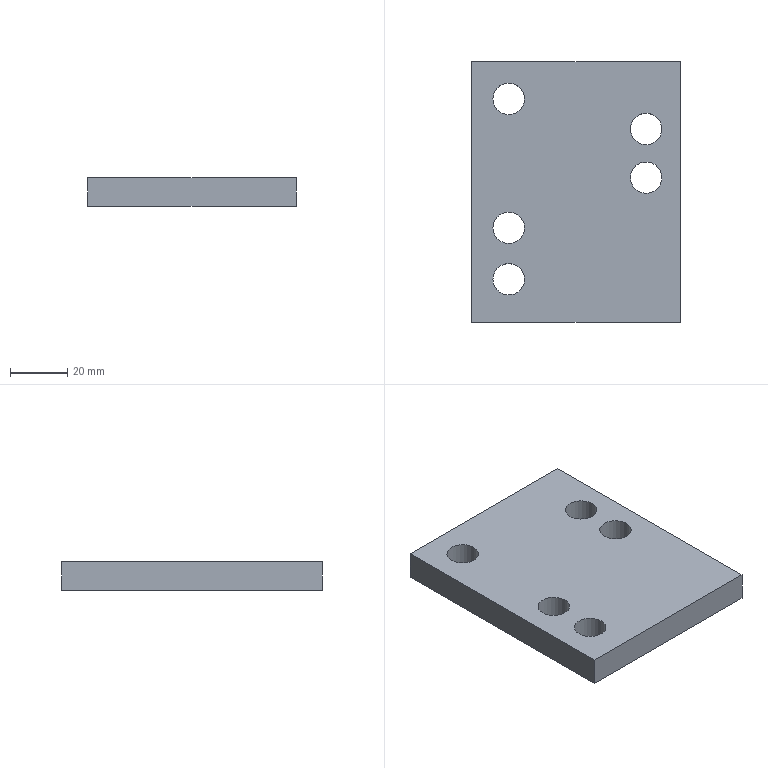Part | NX | features solid 2 | 1 solid | 11 faces | box 73 x 91 x 10 mm | volume 61678 mm3 | plane 6 | cylinder 5 | commonest cylinder face diameters 11 x5
STEP:
#1=CARTESIAN_POINT('',(139.,-184.5,88.));
#2=VERTEX_POINT('',#1);
#3=CARTESIAN_POINT('',(133.5,-184.5,88.));
#4=DIRECTION('',(0.,0.,1.));
#5=DIRECTION('',(1.,0.,0.));
#6=AXIS2_PLACEMENT_3D('',#3,#4,#5);
#7=CIRCLE('',#6,5.5);
#8=EDGE_CURVE('',#2,#2,#7,.T.);
#9=ORIENTED_EDGE('',*,*,#8,.F.);
#10=EDGE_LOOP('',(#9));
#11=FACE_BOUND('',#10,.T.);
#12=CARTESIAN_POINT('',(139.,-166.5,88.));
#13=VERTEX_POINT('',#12);
#14=CARTESIAN_POINT('',(133.5,-166.5,88.));
#15=DIRECTION('',(0.,0.,1.));
#16=DIRECTION('',(1.,0.,0.));
#17=AXIS2_PLACEMENT_3D('',#14,#15,#16);
#18=CIRCLE('',#17,5.5);
#19=EDGE_CURVE('',#13,#13,#18,.T.);
#20=ORIENTED_EDGE('',*,*,#19,.F.);
#21=EDGE_LOOP('',(#20));
#22=FACE_BOUND('',#21,.T.);
#23=CARTESIAN_POINT('',(187.,-132.,88.));
#24=VERTEX_POINT('',#23);
#25=CARTESIAN_POINT('',(181.5,-132.,88.));
#26=DIRECTION('',(0.,0.,1.));
#27=DIRECTION('',(1.,0.,0.));
#28=AXIS2_PLACEMENT_3D('',#25,#26,#27);
#29=CIRCLE('',#28,5.5);
#30=EDGE_CURVE('',#24,#24,#29,.T.);
#31=ORIENTED_EDGE('',*,*,#30,.F.);
#32=EDGE_LOOP('',(#31));
#33=FACE_BOUND('',#32,.T.);
#34=CARTESIAN_POINT('',(139.,-121.5,88.));
#35=VERTEX_POINT('',#34);
#36=CARTESIAN_POINT('',(133.5,-121.5,88.));
#37=DIRECTION('',(0.,0.,1.));
#38=DIRECTION('',(1.,0.,0.));
#39=AXIS2_PLACEMENT_3D('',#36,#37,#38);
#40=CIRCLE('',#39,5.5);
#41=EDGE_CURVE('',#35,#35,#40,.T.);
#42=ORIENTED_EDGE('',*,*,#41,.F.);
#43=EDGE_LOOP('',(#42));
#44=FACE_BOUND('',#43,.T.);
#45=CARTESIAN_POINT('',(187.,-149.,88.));
#46=VERTEX_POINT('',#45);
#47=CARTESIAN_POINT('',(181.5,-149.,88.));
#48=DIRECTION('',(0.,0.,1.));
#49=DIRECTION('',(1.,0.,0.));
#50=AXIS2_PLACEMENT_3D('',#47,#48,#49);
#51=CIRCLE('',#50,5.5);
#52=EDGE_CURVE('',#46,#46,#51,.T.);
#53=ORIENTED_EDGE('',*,*,#52,.F.);
#54=EDGE_LOOP('',(#53));
#55=FACE_BOUND('',#54,.T.);
#56=CARTESIAN_POINT('',(193.5,-199.5,88.));
#57=VERTEX_POINT('',#56);
#58=CARTESIAN_POINT('',(120.5,-199.5,88.));
#59=VERTEX_POINT('',#58);
#60=CARTESIAN_POINT('',(149.,-199.5,88.));
#61=DIRECTION('',(-1.,0.,0.));
#62=VECTOR('',#61,1000.);
#63=LINE('',#60,#62);
#64=EDGE_CURVE('',#57,#59,#63,.T.);
#65=ORIENTED_EDGE('',*,*,#64,.F.);
#66=CARTESIAN_POINT('',(193.5,-108.5,88.));
#67=VERTEX_POINT('',#66);
#68=CARTESIAN_POINT('',(193.5,-140.,88.));
#69=DIRECTION('',(0.,-1.,0.));
#70=VECTOR('',#69,1000.);
#71=LINE('',#68,#70);
#72=EDGE_CURVE('',#67,#57,#71,.T.);
#73=ORIENTED_EDGE('',*,*,#72,.F.);
#74=CARTESIAN_POINT('',(120.5,-108.5,88.));
#75=VERTEX_POINT('',#74);
#76=CARTESIAN_POINT('',(149.,-108.5,88.));
#77=DIRECTION('',(1.,0.,0.));
#78=VECTOR('',#77,1000.);
#79=LINE('',#76,#78);
#80=EDGE_CURVE('',#75,#67,#79,.T.);
#81=ORIENTED_EDGE('',*,*,#80,.F.);
#82=CARTESIAN_POINT('',(120.5,-140.,88.));
#83=DIRECTION('',(0.,1.,0.));
#84=VECTOR('',#83,1000.);
#85=LINE('',#82,#84);
#86=EDGE_CURVE('',#59,#75,#85,.T.);
#87=ORIENTED_EDGE('',*,*,#86,.F.);
#88=EDGE_LOOP('',(#65,#73,#81,#87));
#89=FACE_BOUND('',#88,.T.);
#90=CARTESIAN_POINT('',(268.879,0.,88.));
#91=DIRECTION('',(0.,0.,1.));
#92=DIRECTION('',(-1.,0.,0.));
#93=AXIS2_PLACEMENT_3D('',#90,#91,#92);
#94=PLANE('',#93);
#95=ADVANCED_FACE('',(#11,#22,#33,#44,#55,#89),#94,.T.);
#96=CARTESIAN_POINT('',(193.5,-199.5,78.));
#97=VERTEX_POINT('',#96);
#98=CARTESIAN_POINT('',(193.5,-199.5,19.));
#99=DIRECTION('',(0.,0.,1.));
#100=VECTOR('',#99,1000.);
#101=LINE('',#98,#100);
#102=EDGE_CURVE('',#97,#57,#101,.T.);
#103=ORIENTED_EDGE('',*,*,#102,.T.);
#104=ORIENTED_EDGE('',*,*,#64,.T.);
#105=CARTESIAN_POINT('',(120.5,-199.5,78.));
#106=VERTEX_POINT('',#105);
#107=CARTESIAN_POINT('',(120.5,-199.5,19.));
#108=DIRECTION('',(0.,0.,1.));
#109=VECTOR('',#108,1000.);
#110=LINE('',#107,#109);
#111=EDGE_CURVE('',#106,#59,#110,.T.);
#112=ORIENTED_EDGE('',*,*,#111,.F.);
#113=CARTESIAN_POINT('',(149.,-199.5,78.));
#114=DIRECTION('',(1.,0.,0.));
#115=VECTOR('',#114,1000.);
#116=LINE('',#113,#115);
#117=EDGE_CURVE('',#106,#97,#116,.T.);
#118=ORIENTED_EDGE('',*,*,#117,.T.);
#119=EDGE_LOOP('',(#103,#104,#112,#118));
#120=FACE_BOUND('',#119,.T.);
#121=CARTESIAN_POINT('',(149.,-199.5,19.));
#122=DIRECTION('',(0.,-1.,0.));
#123=DIRECTION('',(0.,0.,-1.));
#124=AXIS2_PLACEMENT_3D('',#121,#122,#123);
#125=PLANE('',#124);
#126=ADVANCED_FACE('',(#120),#125,.T.);
#127=ORIENTED_EDGE('',*,*,#111,.T.);
#128=ORIENTED_EDGE('',*,*,#86,.T.);
#129=CARTESIAN_POINT('',(120.5,-108.5,78.));
#130=VERTEX_POINT('',#129);
#131=CARTESIAN_POINT('',(120.5,-108.5,19.));
#132=DIRECTION('',(0.,0.,1.));
#133=VECTOR('',#132,1000.);
#134=LINE('',#131,#133);
#135=EDGE_CURVE('',#130,#75,#134,.T.);
#136=ORIENTED_EDGE('',*,*,#135,.F.);
#137=CARTESIAN_POINT('',(120.5,-140.,78.));
#138=DIRECTION('',(0.,-1.,0.));
#139=VECTOR('',#138,1000.);
#140=LINE('',#137,#139);
#141=EDGE_CURVE('',#130,#106,#140,.T.);
#142=ORIENTED_EDGE('',*,*,#141,.T.);
#143=EDGE_LOOP('',(#127,#128,#136,#142));
#144=FACE_BOUND('',#143,.T.);
#145=CARTESIAN_POINT('',(120.5,-140.,19.));
#146=DIRECTION('',(-1.,0.,0.));
#147=DIRECTION('',(0.,0.,1.));
#148=AXIS2_PLACEMENT_3D('',#145,#146,#147);
#149=PLANE('',#148);
#150=ADVANCED_FACE('',(#144),#149,.T.);
#151=ORIENTED_EDGE('',*,*,#135,.T.);
#152=ORIENTED_EDGE('',*,*,#80,.T.);
#153=CARTESIAN_POINT('',(193.5,-108.5,78.));
#154=VERTEX_POINT('',#153);
#155=CARTESIAN_POINT('',(193.5,-108.5,19.));
#156=DIRECTION('',(0.,0.,1.));
#157=VECTOR('',#156,1000.);
#158=LINE('',#155,#157);
#159=EDGE_CURVE('',#154,#67,#158,.T.);
#160=ORIENTED_EDGE('',*,*,#159,.F.);
#161=CARTESIAN_POINT('',(149.,-108.5,78.));
#162=DIRECTION('',(-1.,0.,0.));
#163=VECTOR('',#162,1000.);
#164=LINE('',#161,#163);
#165=EDGE_CURVE('',#154,#130,#164,.T.);
#166=ORIENTED_EDGE('',*,*,#165,.T.);
#167=EDGE_LOOP('',(#151,#152,#160,#166));
#168=FACE_BOUND('',#167,.T.);
#169=CARTESIAN_POINT('',(149.,-108.5,19.));
#170=DIRECTION('',(0.,1.,0.));
#171=DIRECTION('',(0.,0.,1.));
#172=AXIS2_PLACEMENT_3D('',#169,#170,#171);
#173=PLANE('',#172);
#174=ADVANCED_FACE('',(#168),#173,.T.);
#175=CARTESIAN_POINT('',(139.,-184.5,78.));
#176=VERTEX_POINT('',#175);
#177=CARTESIAN_POINT('',(133.5,-184.5,78.));
#178=DIRECTION('',(0.,0.,1.));
#179=DIRECTION('',(1.,0.,0.));
#180=AXIS2_PLACEMENT_3D('',#177,#178,#179);
#181=CIRCLE('',#180,5.5);
#182=EDGE_CURVE('',#176,#176,#181,.T.);
#183=ORIENTED_EDGE('',*,*,#182,.T.);
#184=EDGE_LOOP('',(#183));
#185=FACE_BOUND('',#184,.T.);
#186=CARTESIAN_POINT('',(139.,-166.5,78.));
#187=VERTEX_POINT('',#186);
#188=CARTESIAN_POINT('',(133.5,-166.5,78.));
#189=DIRECTION('',(0.,0.,1.));
#190=DIRECTION('',(1.,0.,0.));
#191=AXIS2_PLACEMENT_3D('',#188,#189,#190);
#192=CIRCLE('',#191,5.5);
#193=EDGE_CURVE('',#187,#187,#192,.T.);
#194=ORIENTED_EDGE('',*,*,#193,.T.);
#195=EDGE_LOOP('',(#194));
#196=FACE_BOUND('',#195,.T.);
#197=CARTESIAN_POINT('',(187.,-132.,78.));
#198=VERTEX_POINT('',#197);
#199=CARTESIAN_POINT('',(181.5,-132.,78.));
#200=DIRECTION('',(0.,0.,1.));
#201=DIRECTION('',(1.,0.,0.));
#202=AXIS2_PLACEMENT_3D('',#199,#200,#201);
#203=CIRCLE('',#202,5.5);
#204=EDGE_CURVE('',#198,#198,#203,.T.);
#205=ORIENTED_EDGE('',*,*,#204,.T.);
#206=EDGE_LOOP('',(#205));
#207=FACE_BOUND('',#206,.T.);
#208=CARTESIAN_POINT('',(139.,-121.5,78.));
#209=VERTEX_POINT('',#208);
#210=CARTESIAN_POINT('',(133.5,-121.5,78.));
#211=DIRECTION('',(0.,0.,1.));
#212=DIRECTION('',(1.,0.,0.));
#213=AXIS2_PLACEMENT_3D('',#210,#211,#212);
#214=CIRCLE('',#213,5.5);
#215=EDGE_CURVE('',#209,#209,#214,.T.);
#216=ORIENTED_EDGE('',*,*,#215,.T.);
#217=EDGE_LOOP('',(#216));
#218=FACE_BOUND('',#217,.T.);
#219=CARTESIAN_POINT('',(187.,-149.,78.));
#220=VERTEX_POINT('',#219);
#221=CARTESIAN_POINT('',(181.5,-149.,78.));
#222=DIRECTION('',(0.,0.,1.));
#223=DIRECTION('',(1.,0.,0.));
#224=AXIS2_PLACEMENT_3D('',#221,#222,#223);
#225=CIRCLE('',#224,5.5);
#226=EDGE_CURVE('',#220,#220,#225,.T.);
#227=ORIENTED_EDGE('',*,*,#226,.T.);
#228=EDGE_LOOP('',(#227));
#229=FACE_BOUND('',#228,.T.);
#230=CARTESIAN_POINT('',(193.5,-140.,78.));
#231=DIRECTION('',(0.,1.,0.));
#232=VECTOR('',#231,1000.);
#233=LINE('',#230,#232);
#234=EDGE_CURVE('',#97,#154,#233,.T.);
#235=ORIENTED_EDGE('',*,*,#234,.F.);
#236=ORIENTED_EDGE('',*,*,#117,.F.);
#237=ORIENTED_EDGE('',*,*,#141,.F.);
#238=ORIENTED_EDGE('',*,*,#165,.F.);
#239=EDGE_LOOP('',(#235,#236,#237,#238));
#240=FACE_BOUND('',#239,.T.);
#241=CARTESIAN_POINT('',(149.,-140.,78.));
#242=DIRECTION('',(0.,0.,-1.));
#243=DIRECTION('',(-1.,0.,0.));
#244=AXIS2_PLACEMENT_3D('',#241,#242,#243);
#245=PLANE('',#244);
#246=ADVANCED_FACE('',(#185,#196,#207,#218,#229,#240),#245,.T.);
#247=ORIENTED_EDGE('',*,*,#234,.T.);
#248=ORIENTED_EDGE('',*,*,#159,.T.);
#249=ORIENTED_EDGE('',*,*,#72,.T.);
#250=ORIENTED_EDGE('',*,*,#102,.F.);
#251=EDGE_LOOP('',(#247,#248,#249,#250));
#252=FACE_BOUND('',#251,.T.);
#253=CARTESIAN_POINT('',(193.5,-140.,19.));
#254=DIRECTION('',(1.,0.,0.));
#255=DIRECTION('',(0.,0.,-1.));
#256=AXIS2_PLACEMENT_3D('',#253,#254,#255);
#257=PLANE('',#256);
#258=ADVANCED_FACE('',(#252),#257,.T.);
#259=ORIENTED_EDGE('',*,*,#52,.T.);
#260=EDGE_LOOP('',(#259));
#261=FACE_BOUND('',#260,.T.);
#262=ORIENTED_EDGE('',*,*,#226,.F.);
#263=EDGE_LOOP('',(#262));
#264=FACE_BOUND('',#263,.T.);
#265=CARTESIAN_POINT('',(181.5,-149.,78.));
#266=DIRECTION('',(0.,0.,1.));
#267=DIRECTION('',(1.,0.,0.));
#268=AXIS2_PLACEMENT_3D('',#265,#266,#267);
#269=CYLINDRICAL_SURFACE('',#268,5.5);
#270=ADVANCED_FACE('',(#261,#264),#269,.F.);
#271=ORIENTED_EDGE('',*,*,#41,.T.);
#272=EDGE_LOOP('',(#271));
#273=FACE_BOUND('',#272,.T.);
#274=ORIENTED_EDGE('',*,*,#215,.F.);
#275=EDGE_LOOP('',(#274));
#276=FACE_BOUND('',#275,.T.);
#277=CARTESIAN_POINT('',(133.5,-121.5,78.));
#278=DIRECTION('',(0.,0.,1.));
#279=DIRECTION('',(1.,0.,0.));
#280=AXIS2_PLACEMENT_3D('',#277,#278,#279);
#281=CYLINDRICAL_SURFACE('',#280,5.5);
#282=ADVANCED_FACE('',(#273,#276),#281,.F.);
#283=ORIENTED_EDGE('',*,*,#30,.T.);
#284=EDGE_LOOP('',(#283));
#285=FACE_BOUND('',#284,.T.);
#286=ORIENTED_EDGE('',*,*,#204,.F.);
#287=EDGE_LOOP('',(#286));
#288=FACE_BOUND('',#287,.T.);
#289=CARTESIAN_POINT('',(181.5,-132.,78.));
#290=DIRECTION('',(0.,0.,1.));
#291=DIRECTION('',(1.,0.,0.));
#292=AXIS2_PLACEMENT_3D('',#289,#290,#291);
#293=CYLINDRICAL_SURFACE('',#292,5.5);
#294=ADVANCED_FACE('',(#285,#288),#293,.F.);
#295=ORIENTED_EDGE('',*,*,#19,.T.);
#296=EDGE_LOOP('',(#295));
#297=FACE_BOUND('',#296,.T.);
#298=ORIENTED_EDGE('',*,*,#193,.F.);
#299=EDGE_LOOP('',(#298));
#300=FACE_BOUND('',#299,.T.);
#301=CARTESIAN_POINT('',(133.5,-166.5,78.));
#302=DIRECTION('',(0.,0.,1.));
#303=DIRECTION('',(1.,0.,0.));
#304=AXIS2_PLACEMENT_3D('',#301,#302,#303);
#305=CYLINDRICAL_SURFACE('',#304,5.5);
#306=ADVANCED_FACE('',(#297,#300),#305,.F.);
#307=ORIENTED_EDGE('',*,*,#8,.T.);
#308=EDGE_LOOP('',(#307));
#309=FACE_BOUND('',#308,.T.);
#310=ORIENTED_EDGE('',*,*,#182,.F.);
#311=EDGE_LOOP('',(#310));
#312=FACE_BOUND('',#311,.T.);
#313=CARTESIAN_POINT('',(133.5,-184.5,78.));
#314=DIRECTION('',(0.,0.,1.));
#315=DIRECTION('',(1.,0.,0.));
#316=AXIS2_PLACEMENT_3D('',#313,#314,#315);
#317=CYLINDRICAL_SURFACE('',#316,5.5);
#318=ADVANCED_FACE('',(#309,#312),#317,.F.);
#319=CLOSED_SHELL('',(#95,#126,#150,#174,#246,#258,#270,#282,#294,#306,#318));
#320=MANIFOLD_SOLID_BREP('',#319);
#321=(LENGTH_UNIT()NAMED_UNIT(*)SI_UNIT(.MILLI.,.METRE.));
#322=UNCERTAINTY_MEASURE_WITH_UNIT(LENGTH_MEASURE(0.00001),#321,'','');
#323=(NAMED_UNIT(*)PLANE_ANGLE_UNIT()SI_UNIT($,.RADIAN.));
#324=(NAMED_UNIT(*)SI_UNIT($,.STERADIAN.)SOLID_ANGLE_UNIT());
#325=(GEOMETRIC_REPRESENTATION_CONTEXT(3)GLOBAL_UNCERTAINTY_ASSIGNED_CONTEXT((#322))GLOBAL_UNIT_ASSIGNED_CONTEXT((#321,#323,#324))REPRESENTATION_CONTEXT('',''));
#326=ADVANCED_BREP_SHAPE_REPRESENTATION('',(#320),#325);